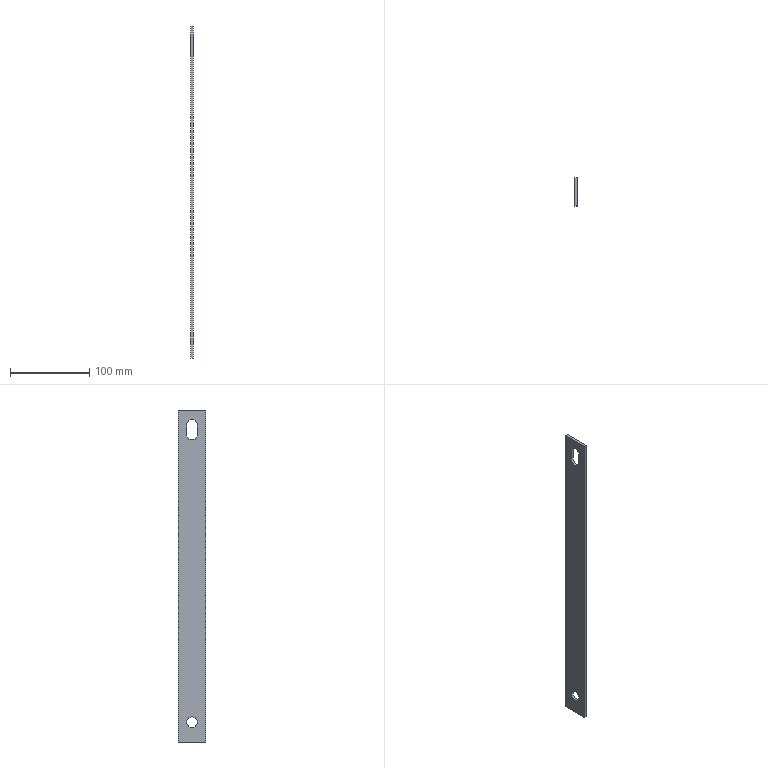Part | NX | features solid 2 | 1 solid | 11 faces | box 3 x 35 x 420 mm | volume 42735 mm3 | plane 8 | cylinder 3 | commonest cylinder face diameters 13.5 x3
STEP:
#1=CARTESIAN_POINT('',(1635.,493.25,351.25));
#2=VERTEX_POINT('',#1);
#3=CARTESIAN_POINT('',(1635.,506.75,351.25));
#4=VERTEX_POINT('',#3);
#5=CARTESIAN_POINT('',(1635.,500.,351.25));
#6=DIRECTION('',(-1.,0.,0.));
#7=DIRECTION('',(0.,-1.,0.));
#8=AXIS2_PLACEMENT_3D('',#5,#6,#7);
#9=CIRCLE('',#8,6.75);
#10=EDGE_CURVE('',#2,#4,#9,.T.);
#11=ORIENTED_EDGE('',*,*,#10,.T.);
#12=CARTESIAN_POINT('',(1638.,506.75,351.25));
#13=VERTEX_POINT('',#12);
#14=CARTESIAN_POINT('',(1638.,506.75,351.25));
#15=DIRECTION('',(-1.,0.,0.));
#16=VECTOR('',#15,1000.);
#17=LINE('',#14,#16);
#18=EDGE_CURVE('',#13,#4,#17,.T.);
#19=ORIENTED_EDGE('',*,*,#18,.F.);
#20=CARTESIAN_POINT('',(1638.,493.25,351.25));
#21=VERTEX_POINT('',#20);
#22=CARTESIAN_POINT('',(1638.,500.,351.25));
#23=DIRECTION('',(-1.,0.,0.));
#24=DIRECTION('',(0.,-1.,0.));
#25=AXIS2_PLACEMENT_3D('',#22,#23,#24);
#26=CIRCLE('',#25,6.75);
#27=EDGE_CURVE('',#21,#13,#26,.T.);
#28=ORIENTED_EDGE('',*,*,#27,.F.);
#29=CARTESIAN_POINT('',(1638.,493.25,351.25));
#30=DIRECTION('',(-1.,0.,0.));
#31=VECTOR('',#30,1000.);
#32=LINE('',#29,#31);
#33=EDGE_CURVE('',#21,#2,#32,.T.);
#34=ORIENTED_EDGE('',*,*,#33,.T.);
#35=EDGE_LOOP('',(#11,#19,#28,#34));
#36=FACE_BOUND('',#35,.T.);
#37=CARTESIAN_POINT('',(1638.,500.,351.25));
#38=DIRECTION('',(-1.,0.,0.));
#39=DIRECTION('',(0.,-1.,0.));
#40=AXIS2_PLACEMENT_3D('',#37,#38,#39);
#41=CYLINDRICAL_SURFACE('',#40,6.75);
#42=ADVANCED_FACE('',(#36),#41,.F.);
#43=CARTESIAN_POINT('',(1635.,493.25,338.75));
#44=VERTEX_POINT('',#43);
#45=CARTESIAN_POINT('',(1635.,493.25,351.25));
#46=DIRECTION('',(0.,0.,-1.));
#47=VECTOR('',#46,1000.);
#48=LINE('',#45,#47);
#49=EDGE_CURVE('',#2,#44,#48,.T.);
#50=ORIENTED_EDGE('',*,*,#49,.F.);
#51=ORIENTED_EDGE('',*,*,#33,.F.);
#52=CARTESIAN_POINT('',(1638.,493.25,338.75));
#53=VERTEX_POINT('',#52);
#54=CARTESIAN_POINT('',(1638.,493.25,351.25));
#55=DIRECTION('',(0.,0.,-1.));
#56=VECTOR('',#55,1000.);
#57=LINE('',#54,#56);
#58=EDGE_CURVE('',#21,#53,#57,.T.);
#59=ORIENTED_EDGE('',*,*,#58,.T.);
#60=CARTESIAN_POINT('',(1638.,493.25,338.75));
#61=DIRECTION('',(-1.,0.,0.));
#62=VECTOR('',#61,1000.);
#63=LINE('',#60,#62);
#64=EDGE_CURVE('',#53,#44,#63,.T.);
#65=ORIENTED_EDGE('',*,*,#64,.T.);
#66=EDGE_LOOP('',(#50,#51,#59,#65));
#67=FACE_BOUND('',#66,.T.);
#68=CARTESIAN_POINT('',(1638.,493.25,351.25));
#69=DIRECTION('',(0.,1.,0.));
#70=DIRECTION('',(-1.,0.,0.));
#71=AXIS2_PLACEMENT_3D('',#68,#69,#70);
#72=PLANE('',#71);
#73=ADVANCED_FACE('',(#67),#72,.T.);
#74=CARTESIAN_POINT('',(1635.,506.75,338.75));
#75=VERTEX_POINT('',#74);
#76=CARTESIAN_POINT('',(1635.,500.,338.75));
#77=DIRECTION('',(-1.,0.,0.));
#78=DIRECTION('',(0.,-1.,0.));
#79=AXIS2_PLACEMENT_3D('',#76,#77,#78);
#80=CIRCLE('',#79,6.75);
#81=EDGE_CURVE('',#75,#44,#80,.T.);
#82=ORIENTED_EDGE('',*,*,#81,.T.);
#83=ORIENTED_EDGE('',*,*,#64,.F.);
#84=CARTESIAN_POINT('',(1638.,506.75,338.75));
#85=VERTEX_POINT('',#84);
#86=CARTESIAN_POINT('',(1638.,500.,338.75));
#87=DIRECTION('',(-1.,0.,0.));
#88=DIRECTION('',(0.,-1.,0.));
#89=AXIS2_PLACEMENT_3D('',#86,#87,#88);
#90=CIRCLE('',#89,6.75);
#91=EDGE_CURVE('',#85,#53,#90,.T.);
#92=ORIENTED_EDGE('',*,*,#91,.F.);
#93=CARTESIAN_POINT('',(1638.,506.75,338.75));
#94=DIRECTION('',(-1.,0.,0.));
#95=VECTOR('',#94,1000.);
#96=LINE('',#93,#95);
#97=EDGE_CURVE('',#85,#75,#96,.T.);
#98=ORIENTED_EDGE('',*,*,#97,.T.);
#99=EDGE_LOOP('',(#82,#83,#92,#98));
#100=FACE_BOUND('',#99,.T.);
#101=CARTESIAN_POINT('',(1638.,500.,338.75));
#102=DIRECTION('',(-1.,0.,0.));
#103=DIRECTION('',(0.,-1.,0.));
#104=AXIS2_PLACEMENT_3D('',#101,#102,#103);
#105=CYLINDRICAL_SURFACE('',#104,6.75);
#106=ADVANCED_FACE('',(#100),#105,.F.);
#107=CARTESIAN_POINT('',(1635.,482.5,-50.));
#108=VERTEX_POINT('',#107);
#109=CARTESIAN_POINT('',(1635.,482.5,370.));
#110=VERTEX_POINT('',#109);
#111=CARTESIAN_POINT('',(1635.,482.5,70.));
#112=DIRECTION('',(0.,0.,1.));
#113=VECTOR('',#112,1000.);
#114=LINE('',#111,#113);
#115=EDGE_CURVE('',#108,#110,#114,.T.);
#116=ORIENTED_EDGE('',*,*,#115,.F.);
#117=CARTESIAN_POINT('',(1638.,482.5,-50.));
#118=VERTEX_POINT('',#117);
#119=CARTESIAN_POINT('',(1638.,482.5,-50.));
#120=DIRECTION('',(-1.,0.,0.));
#121=VECTOR('',#120,1000.);
#122=LINE('',#119,#121);
#123=EDGE_CURVE('',#118,#108,#122,.T.);
#124=ORIENTED_EDGE('',*,*,#123,.F.);
#125=CARTESIAN_POINT('',(1638.,482.5,370.));
#126=VERTEX_POINT('',#125);
#127=CARTESIAN_POINT('',(1638.,482.5,70.));
#128=DIRECTION('',(0.,0.,1.));
#129=VECTOR('',#128,1000.);
#130=LINE('',#127,#129);
#131=EDGE_CURVE('',#118,#126,#130,.T.);
#132=ORIENTED_EDGE('',*,*,#131,.T.);
#133=CARTESIAN_POINT('',(1638.,482.5,370.));
#134=DIRECTION('',(-1.,0.,0.));
#135=VECTOR('',#134,1000.);
#136=LINE('',#133,#135);
#137=EDGE_CURVE('',#126,#110,#136,.T.);
#138=ORIENTED_EDGE('',*,*,#137,.T.);
#139=EDGE_LOOP('',(#116,#124,#132,#138));
#140=FACE_BOUND('',#139,.T.);
#141=CARTESIAN_POINT('',(1638.,482.5,70.));
#142=DIRECTION('',(0.,-1.,0.));
#143=DIRECTION('',(0.,0.,1.));
#144=AXIS2_PLACEMENT_3D('',#141,#142,#143);
#145=PLANE('',#144);
#146=ADVANCED_FACE('',(#140),#145,.T.);
#147=CARTESIAN_POINT('',(1635.,517.5,370.));
#148=VERTEX_POINT('',#147);
#149=CARTESIAN_POINT('',(1635.,482.5,370.));
#150=DIRECTION('',(0.,1.,0.));
#151=VECTOR('',#150,1000.);
#152=LINE('',#149,#151);
#153=EDGE_CURVE('',#110,#148,#152,.T.);
#154=ORIENTED_EDGE('',*,*,#153,.F.);
#155=ORIENTED_EDGE('',*,*,#137,.F.);
#156=CARTESIAN_POINT('',(1638.,517.5,370.));
#157=VERTEX_POINT('',#156);
#158=CARTESIAN_POINT('',(1638.,482.5,370.));
#159=DIRECTION('',(0.,1.,0.));
#160=VECTOR('',#159,1000.);
#161=LINE('',#158,#160);
#162=EDGE_CURVE('',#126,#157,#161,.T.);
#163=ORIENTED_EDGE('',*,*,#162,.T.);
#164=CARTESIAN_POINT('',(1638.,517.5,370.));
#165=DIRECTION('',(-1.,0.,0.));
#166=VECTOR('',#165,1000.);
#167=LINE('',#164,#166);
#168=EDGE_CURVE('',#157,#148,#167,.T.);
#169=ORIENTED_EDGE('',*,*,#168,.T.);
#170=EDGE_LOOP('',(#154,#155,#163,#169));
#171=FACE_BOUND('',#170,.T.);
#172=CARTESIAN_POINT('',(1638.,482.5,370.));
#173=DIRECTION('',(0.,0.,1.));
#174=DIRECTION('',(-1.,0.,0.));
#175=AXIS2_PLACEMENT_3D('',#172,#173,#174);
#176=PLANE('',#175);
#177=ADVANCED_FACE('',(#171),#176,.T.);
#178=CARTESIAN_POINT('',(1635.,517.5,-50.));
#179=VERTEX_POINT('',#178);
#180=CARTESIAN_POINT('',(1635.,517.5,370.));
#181=DIRECTION('',(0.,0.,-1.));
#182=VECTOR('',#181,1000.);
#183=LINE('',#180,#182);
#184=EDGE_CURVE('',#148,#179,#183,.T.);
#185=ORIENTED_EDGE('',*,*,#184,.F.);
#186=ORIENTED_EDGE('',*,*,#168,.F.);
#187=CARTESIAN_POINT('',(1638.,517.5,-50.));
#188=VERTEX_POINT('',#187);
#189=CARTESIAN_POINT('',(1638.,517.5,370.));
#190=DIRECTION('',(0.,0.,-1.));
#191=VECTOR('',#190,1000.);
#192=LINE('',#189,#191);
#193=EDGE_CURVE('',#157,#188,#192,.T.);
#194=ORIENTED_EDGE('',*,*,#193,.T.);
#195=CARTESIAN_POINT('',(1638.,517.5,-50.));
#196=DIRECTION('',(-1.,0.,0.));
#197=VECTOR('',#196,1000.);
#198=LINE('',#195,#197);
#199=EDGE_CURVE('',#188,#179,#198,.T.);
#200=ORIENTED_EDGE('',*,*,#199,.T.);
#201=EDGE_LOOP('',(#185,#186,#194,#200));
#202=FACE_BOUND('',#201,.T.);
#203=CARTESIAN_POINT('',(1638.,517.5,370.));
#204=DIRECTION('',(0.,1.,0.));
#205=DIRECTION('',(0.,0.,-1.));
#206=AXIS2_PLACEMENT_3D('',#203,#204,#205);
#207=PLANE('',#206);
#208=ADVANCED_FACE('',(#202),#207,.T.);
#209=CARTESIAN_POINT('',(1638.,493.25,-25.));
#210=VERTEX_POINT('',#209);
#211=CARTESIAN_POINT('',(1638.,500.,-25.));
#212=DIRECTION('',(-1.,0.,0.));
#213=DIRECTION('',(0.,-1.,0.));
#214=AXIS2_PLACEMENT_3D('',#211,#212,#213);
#215=CIRCLE('',#214,6.75);
#216=EDGE_CURVE('',#210,#210,#215,.T.);
#217=ORIENTED_EDGE('',*,*,#216,.F.);
#218=EDGE_LOOP('',(#217));
#219=FACE_BOUND('',#218,.T.);
#220=CARTESIAN_POINT('',(1635.,493.25,-25.));
#221=VERTEX_POINT('',#220);
#222=CARTESIAN_POINT('',(1635.,500.,-25.));
#223=DIRECTION('',(-1.,0.,0.));
#224=DIRECTION('',(0.,-1.,0.));
#225=AXIS2_PLACEMENT_3D('',#222,#223,#224);
#226=CIRCLE('',#225,6.75);
#227=EDGE_CURVE('',#221,#221,#226,.T.);
#228=ORIENTED_EDGE('',*,*,#227,.T.);
#229=EDGE_LOOP('',(#228));
#230=FACE_BOUND('',#229,.T.);
#231=CARTESIAN_POINT('',(1638.,500.,-25.));
#232=DIRECTION('',(-1.,0.,0.));
#233=DIRECTION('',(0.,-1.,0.));
#234=AXIS2_PLACEMENT_3D('',#231,#232,#233);
#235=CYLINDRICAL_SURFACE('',#234,6.75);
#236=ADVANCED_FACE('',(#219,#230),#235,.F.);
#237=CARTESIAN_POINT('',(1635.,517.5,-50.));
#238=DIRECTION('',(0.,-1.,0.));
#239=VECTOR('',#238,1000.);
#240=LINE('',#237,#239);
#241=EDGE_CURVE('',#179,#108,#240,.T.);
#242=ORIENTED_EDGE('',*,*,#241,.F.);
#243=ORIENTED_EDGE('',*,*,#199,.F.);
#244=CARTESIAN_POINT('',(1638.,517.5,-50.));
#245=DIRECTION('',(0.,-1.,0.));
#246=VECTOR('',#245,1000.);
#247=LINE('',#244,#246);
#248=EDGE_CURVE('',#188,#118,#247,.T.);
#249=ORIENTED_EDGE('',*,*,#248,.T.);
#250=ORIENTED_EDGE('',*,*,#123,.T.);
#251=EDGE_LOOP('',(#242,#243,#249,#250));
#252=FACE_BOUND('',#251,.T.);
#253=CARTESIAN_POINT('',(1638.,517.5,-50.));
#254=DIRECTION('',(0.,0.,-1.));
#255=DIRECTION('',(1.,0.,0.));
#256=AXIS2_PLACEMENT_3D('',#253,#254,#255);
#257=PLANE('',#256);
#258=ADVANCED_FACE('',(#252),#257,.T.);
#259=CARTESIAN_POINT('',(1635.,506.75,338.75));
#260=DIRECTION('',(0.,0.,1.));
#261=VECTOR('',#260,1000.);
#262=LINE('',#259,#261);
#263=EDGE_CURVE('',#75,#4,#262,.T.);
#264=ORIENTED_EDGE('',*,*,#263,.F.);
#265=ORIENTED_EDGE('',*,*,#97,.F.);
#266=CARTESIAN_POINT('',(1638.,506.75,338.75));
#267=DIRECTION('',(0.,0.,1.));
#268=VECTOR('',#267,1000.);
#269=LINE('',#266,#268);
#270=EDGE_CURVE('',#85,#13,#269,.T.);
#271=ORIENTED_EDGE('',*,*,#270,.T.);
#272=ORIENTED_EDGE('',*,*,#18,.T.);
#273=EDGE_LOOP('',(#264,#265,#271,#272));
#274=FACE_BOUND('',#273,.T.);
#275=CARTESIAN_POINT('',(1638.,506.75,338.75));
#276=DIRECTION('',(0.,-1.,0.));
#277=DIRECTION('',(1.,0.,0.));
#278=AXIS2_PLACEMENT_3D('',#275,#276,#277);
#279=PLANE('',#278);
#280=ADVANCED_FACE('',(#274),#279,.T.);
#281=ORIENTED_EDGE('',*,*,#131,.F.);
#282=ORIENTED_EDGE('',*,*,#248,.F.);
#283=ORIENTED_EDGE('',*,*,#193,.F.);
#284=ORIENTED_EDGE('',*,*,#162,.F.);
#285=EDGE_LOOP('',(#281,#282,#283,#284));
#286=FACE_BOUND('',#285,.T.);
#287=ORIENTED_EDGE('',*,*,#216,.T.);
#288=EDGE_LOOP('',(#287));
#289=FACE_BOUND('',#288,.T.);
#290=ORIENTED_EDGE('',*,*,#27,.T.);
#291=ORIENTED_EDGE('',*,*,#270,.F.);
#292=ORIENTED_EDGE('',*,*,#91,.T.);
#293=ORIENTED_EDGE('',*,*,#58,.F.);
#294=EDGE_LOOP('',(#290,#291,#292,#293));
#295=FACE_BOUND('',#294,.T.);
#296=CARTESIAN_POINT('',(1638.,482.5,370.));
#297=DIRECTION('',(-1.,0.,0.));
#298=DIRECTION('',(0.,-1.,0.));
#299=AXIS2_PLACEMENT_3D('',#296,#297,#298);
#300=PLANE('',#299);
#301=ADVANCED_FACE('',(#286,#289,#295),#300,.F.);
#302=ORIENTED_EDGE('',*,*,#115,.T.);
#303=ORIENTED_EDGE('',*,*,#153,.T.);
#304=ORIENTED_EDGE('',*,*,#184,.T.);
#305=ORIENTED_EDGE('',*,*,#241,.T.);
#306=EDGE_LOOP('',(#302,#303,#304,#305));
#307=FACE_BOUND('',#306,.T.);
#308=ORIENTED_EDGE('',*,*,#227,.F.);
#309=EDGE_LOOP('',(#308));
#310=FACE_BOUND('',#309,.T.);
#311=ORIENTED_EDGE('',*,*,#10,.F.);
#312=ORIENTED_EDGE('',*,*,#49,.T.);
#313=ORIENTED_EDGE('',*,*,#81,.F.);
#314=ORIENTED_EDGE('',*,*,#263,.T.);
#315=EDGE_LOOP('',(#311,#312,#313,#314));
#316=FACE_BOUND('',#315,.T.);
#317=CARTESIAN_POINT('',(1635.,482.5,370.));
#318=DIRECTION('',(-1.,0.,0.));
#319=DIRECTION('',(0.,-1.,0.));
#320=AXIS2_PLACEMENT_3D('',#317,#318,#319);
#321=PLANE('',#320);
#322=ADVANCED_FACE('',(#307,#310,#316),#321,.T.);
#323=CLOSED_SHELL('',(#42,#73,#106,#146,#177,#208,#236,#258,#280,#301,#322));
#324=MANIFOLD_SOLID_BREP('',#323);
#325=(LENGTH_UNIT()NAMED_UNIT(*)SI_UNIT(.MILLI.,.METRE.));
#326=UNCERTAINTY_MEASURE_WITH_UNIT(LENGTH_MEASURE(0.00001),#325,'','');
#327=(NAMED_UNIT(*)PLANE_ANGLE_UNIT()SI_UNIT($,.RADIAN.));
#328=(NAMED_UNIT(*)SI_UNIT($,.STERADIAN.)SOLID_ANGLE_UNIT());
#329=(GEOMETRIC_REPRESENTATION_CONTEXT(3)GLOBAL_UNCERTAINTY_ASSIGNED_CONTEXT((#326))GLOBAL_UNIT_ASSIGNED_CONTEXT((#325,#327,#328))REPRESENTATION_CONTEXT('',''));
#330=ADVANCED_BREP_SHAPE_REPRESENTATION('',(#324),#329);